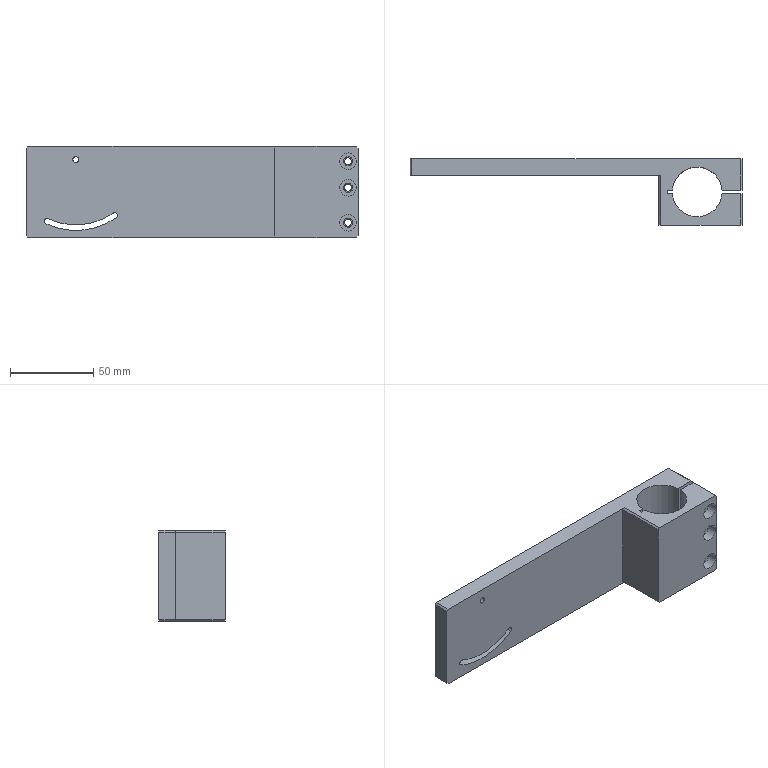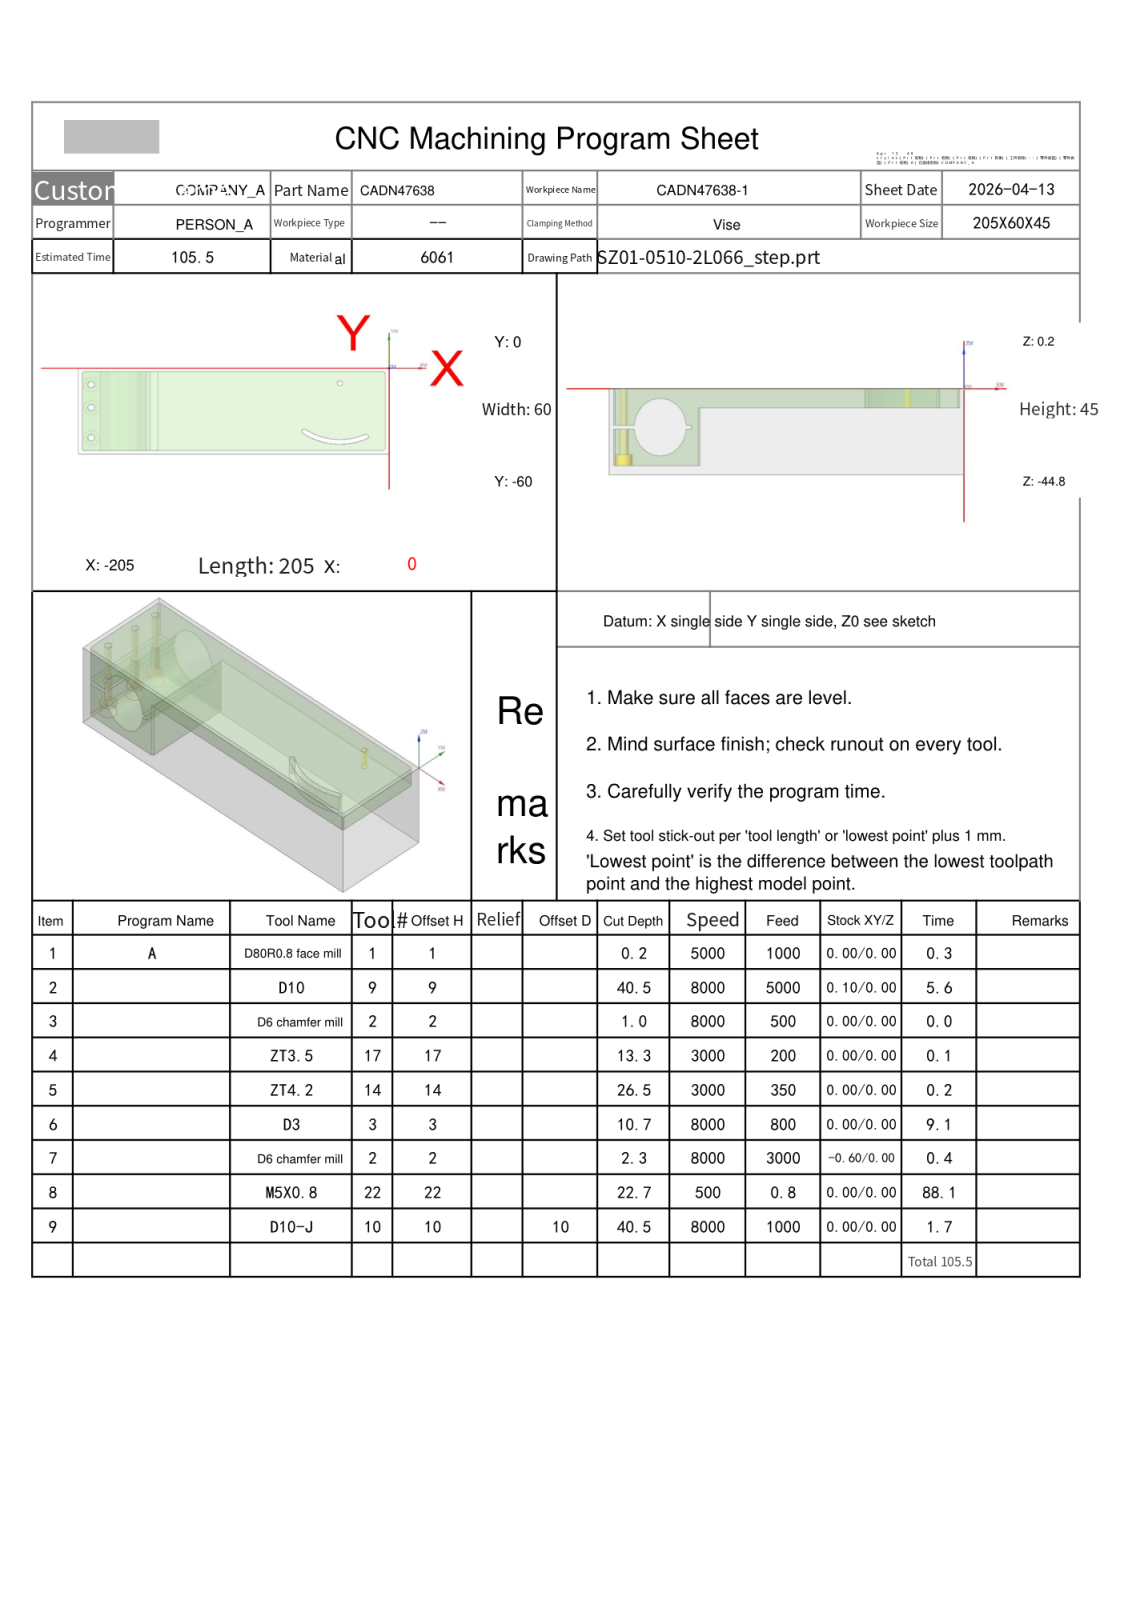NC program | NX | posted by the shop | part box 200 x 40 x 55 mm
Lines 1034 to 2500 of 2500:
N6 T03 M06
(D3  D=3. R=0. H=03 ce=0.10 di=0.00)
(D.N=03 MAX_Z=20. MIN_Z=-10.5 Time=9.14M)
G00 G90 G54 X-36.076 Y-51.374 M03 S8000
G43 H03 Z20.
M08
Z.5
G03 X-15.16 Y-47.686 Z.463 I3.576 J40.874 F800.
G01 X-15.132 Y-47.675
X-15.121 Y-47.646
X-15.136 Y-47.619
X-15.147 Y-47.591
X-15.176 Y-47.581
X-15.202 Y-47.595
G02 X-55.976 Y-44.028 Z.389 I-17.298 J37.095
G01 X-56. Y-44.009
X-56.031 Y-44.014
X-56.046 Y-44.04
X-56.065 Y-44.064
X-56.06 Y-44.094 Z.388
X-56.034 Y-44.11
G03 X-36.076 Y-51.374 Z.351 I23.534 J33.61
X-15.16 Y-47.686 Z.314 I3.576 J40.874
G01 X-15.132 Y-47.675
X-15.121 Y-47.646
X-15.136 Y-47.619
X-15.147 Y-47.591
X-15.176 Y-47.581
X-15.202 Y-47.595
G02 X-55.976 Y-44.028 Z.24 I-17.298 J37.095
G01 X-56. Y-44.009
X-56.031 Y-44.014
X-56.046 Y-44.04
X-56.065 Y-44.064
X-56.06 Y-44.094
X-56.034 Y-44.11
G03 X-36.076 Y-51.374 Z.203 I23.534 J33.61
X-15.16 Y-47.686 Z.166 I3.576 J40.874
G01 X-15.132 Y-47.675
X-15.121 Y-47.646
X-15.136 Y-47.619 Z.165
X-15.147 Y-47.591
X-15.176 Y-47.581
X-15.202 Y-47.595
G02 X-55.976 Y-44.028 Z.091 I-17.298 J37.095
G01 X-56. Y-44.009
X-56.031 Y-44.014
X-56.046 Y-44.04
X-56.065 Y-44.064
X-56.06 Y-44.094
X-56.034 Y-44.11
G03 X-36.076 Y-51.374 Z.054 I23.534 J33.61
X-15.16 Y-47.686 Z.017 I3.576 J40.874
G01 X-15.132 Y-47.675
X-15.121 Y-47.646
X-15.136 Y-47.619
X-15.147 Y-47.591
X-15.176 Y-47.581
X-15.202 Y-47.595
G02 X-55.976 Y-44.028 Z-.057 I-17.298 J37.095
G01 X-56. Y-44.009
X-56.031 Y-44.014
X-56.046 Y-44.04
X-56.065 Y-44.064
X-56.06 Y-44.094
X-56.034 Y-44.11 Z-.058
G03 X-36.076 Y-51.374 Z-.095 I23.534 J33.61
X-15.16 Y-47.686 Z-.132 I3.576 J40.874
G01 X-15.132 Y-47.675
X-15.121 Y-47.646
X-15.136 Y-47.619
X-15.147 Y-47.591
X-15.176 Y-47.581
X-15.202 Y-47.595
G02 X-55.976 Y-44.028 Z-.206 I-17.298 J37.095
G01 X-56. Y-44.009
X-56.031 Y-44.014
X-56.046 Y-44.04
X-56.065 Y-44.064
X-56.06 Y-44.094
X-56.034 Y-44.11
G03 X-36.076 Y-51.374 Z-.243 I23.534 J33.61
X-15.16 Y-47.686 Z-.28 I3.576 J40.874
G01 X-15.132 Y-47.675
X-15.121 Y-47.646
X-15.136 Y-47.619
X-15.147 Y-47.591
X-15.176 Y-47.581 Z-.281
X-15.202 Y-47.595
G02 X-55.976 Y-44.028 Z-.355 I-17.298 J37.095
G01 X-56. Y-44.009
X-56.031 Y-44.014
X-56.046 Y-44.04
X-56.065 Y-44.064
X-56.06 Y-44.094
X-56.034 Y-44.11
G03 X-36.076 Y-51.374 Z-.392 I23.534 J33.61
X-15.16 Y-47.686 Z-.429 I3.576 J40.874
G01 X-15.132 Y-47.675
X-15.121 Y-47.646
X-15.136 Y-47.619
X-15.147 Y-47.591
X-15.176 Y-47.581
X-15.202 Y-47.595
G02 X-55.976 Y-44.028 Z-.503 I-17.298 J37.095
G01 X-56. Y-44.009
X-56.031 Y-44.014
X-56.046 Y-44.04
X-56.065 Y-44.064
X-56.06 Y-44.094
X-56.034 Y-44.11
G03 X-36.076 Y-51.374 Z-.541 I23.534 J33.61
X-15.16 Y-47.686 Z-.578 I3.576 J40.874
G01 X-15.132 Y-47.675
X-15.121 Y-47.646
X-15.136 Y-47.619
X-15.147 Y-47.591
X-15.176 Y-47.581
X-15.202 Y-47.595
G02 X-55.976 Y-44.028 Z-.652 I-17.298 J37.095
G01 X-56. Y-44.009
X-56.031 Y-44.014
X-56.046 Y-44.04
X-56.065 Y-44.064
X-56.06 Y-44.094
X-56.034 Y-44.11
G03 X-36.076 Y-51.374 Z-.689 I23.534 J33.61
X-15.16 Y-47.686 Z-.726 I3.576 J40.874
G01 X-15.132 Y-47.675
X-15.121 Y-47.646
X-15.136 Y-47.619
X-15.147 Y-47.591
X-15.176 Y-47.581
X-15.202 Y-47.595 Z-.727
G02 X-55.976 Y-44.028 Z-.8 I-17.298 J37.095
G01 X-56. Y-44.009 Z-.801
X-56.031 Y-44.014
X-56.046 Y-44.04
X-56.065 Y-44.064
X-56.06 Y-44.094
X-56.034 Y-44.11
G03 X-36.076 Y-51.374 Z-.838 I23.534 J33.61
X-15.16 Y-47.686 Z-.875 I3.576 J40.874
G01 X-15.132 Y-47.675
X-15.121 Y-47.646
X-15.136 Y-47.619
X-15.147 Y-47.591
X-15.176 Y-47.581
X-15.202 Y-47.595
G02 X-55.976 Y-44.028 Z-.949 I-17.298 J37.095
G01 X-56. Y-44.009
X-56.031 Y-44.014
X-56.046 Y-44.04
X-56.065 Y-44.064
X-56.06 Y-44.094
X-56.034 Y-44.11
G03 X-36.076 Y-51.374 Z-.986 I23.534 J33.61
X-15.16 Y-47.686 Z-1.024 I3.576 J40.874
G01 X-15.132 Y-47.675
X-15.121 Y-47.646
X-15.136 Y-47.619
X-15.147 Y-47.591
X-15.176 Y-47.581
X-15.202 Y-47.595
G02 X-55.976 Y-44.028 Z-1.098 I-17.298 J37.095
G01 X-56. Y-44.009
X-56.031 Y-44.014
X-56.046 Y-44.04
X-56.065 Y-44.064
X-56.06 Y-44.094
X-56.034 Y-44.11
G03 X-36.076 Y-51.374 Z-1.135 I23.534 J33.61
X-15.16 Y-47.686 Z-1.172 I3.576 J40.874
G01 X-15.132 Y-47.675
X-15.121 Y-47.646
X-15.136 Y-47.619
X-15.147 Y-47.591
X-15.176 Y-47.581
X-15.202 Y-47.595
G02 X-55.976 Y-44.028 Z-1.246 I-17.298 J37.095
G01 X-56. Y-44.009
X-56.031 Y-44.014 Z-1.247
X-56.046 Y-44.04
X-56.065 Y-44.064
X-56.06 Y-44.094
X-56.034 Y-44.11
G03 X-36.076 Y-51.374 Z-1.284 I23.534 J33.61
X-15.16 Y-47.686 Z-1.321 I3.576 J40.874
G01 X-15.132 Y-47.675
X-15.121 Y-47.646
X-15.136 Y-47.619
X-15.147 Y-47.591
X-15.176 Y-47.581
X-15.202 Y-47.595
G02 X-55.976 Y-44.028 Z-1.395 I-17.298 J37.095
G01 X-56. Y-44.009
X-56.031 Y-44.014
X-56.046 Y-44.04
X-56.065 Y-44.064
X-56.06 Y-44.094
X-56.034 Y-44.11
G03 X-36.076 Y-51.374 Z-1.432 I23.534 J33.61
X-15.16 Y-47.686 Z-1.47 I3.576 J40.874
G01 X-15.132 Y-47.675
X-15.121 Y-47.646
X-15.136 Y-47.619
X-15.147 Y-47.591
X-15.176 Y-47.581
X-15.202 Y-47.595
G02 X-55.976 Y-44.028 Z-1.544 I-17.298 J37.095
G01 X-56. Y-44.009
X-56.031 Y-44.014
X-56.046 Y-44.04
X-56.065 Y-44.064
X-56.06 Y-44.094
X-56.034 Y-44.11
G03 X-36.076 Y-51.374 Z-1.581 I23.534 J33.61
X-15.16 Y-47.686 Z-1.618 I3.576 J40.874
G01 X-15.132 Y-47.675
X-15.121 Y-47.646
X-15.136 Y-47.619
X-15.147 Y-47.591
X-15.176 Y-47.581
X-15.202 Y-47.595
G02 X-55.976 Y-44.028 Z-1.692 I-17.298 J37.095
G01 X-56. Y-44.009
X-56.031 Y-44.014
X-56.046 Y-44.04 Z-1.693
X-56.065 Y-44.064
X-56.06 Y-44.094
X-56.034 Y-44.11
G03 X-36.076 Y-51.374 Z-1.73 I23.534 J33.61
X-15.16 Y-47.686 Z-1.767 I3.576 J40.874
G01 X-15.132 Y-47.675
X-15.121 Y-47.646
X-15.136 Y-47.619
X-15.147 Y-47.591
X-15.176 Y-47.581
X-15.202 Y-47.595
G02 X-55.976 Y-44.028 Z-1.841 I-17.298 J37.095
G01 X-56. Y-44.009
X-56.031 Y-44.014
X-56.046 Y-44.04
X-56.065 Y-44.064
X-56.06 Y-44.094
X-56.034 Y-44.11
G03 X-36.076 Y-51.374 Z-1.878 I23.534 J33.61
X-15.16 Y-47.686 Z-1.915 I3.576 J40.874
G01 X-15.132 Y-47.675
X-15.121 Y-47.646 Z-1.916
X-15.136 Y-47.619
X-15.147 Y-47.591
X-15.176 Y-47.581
X-15.202 Y-47.595
G02 X-55.976 Y-44.028 Z-1.99 I-17.298 J37.095
G01 X-56. Y-44.009
X-56.031 Y-44.014
X-56.046 Y-44.04
X-56.065 Y-44.064
X-56.06 Y-44.094
X-56.034 Y-44.11
G03 X-36.076 Y-51.374 Z-2.027 I23.534 J33.61
X-15.16 Y-47.686 Z-2.064 I3.576 J40.874
G01 X-15.132 Y-47.675
X-15.121 Y-47.646
X-15.136 Y-47.619
X-15.147 Y-47.591
X-15.176 Y-47.581
X-15.202 Y-47.595
G02 X-55.976 Y-44.028 Z-2.138 I-17.298 J37.095
G01 X-56. Y-44.009
X-56.031 Y-44.014
X-56.046 Y-44.04
X-56.065 Y-44.064 Z-2.139
X-56.06 Y-44.094
X-56.034 Y-44.11
G03 X-36.076 Y-51.374 Z-2.176 I23.534 J33.61
X-15.16 Y-47.686 Z-2.213 I3.576 J40.874
G01 X-15.132 Y-47.675
X-15.121 Y-47.646
X-15.136 Y-47.619
X-15.147 Y-47.591
X-15.176 Y-47.581
X-15.202 Y-47.595
G02 X-55.976 Y-44.028 Z-2.287 I-17.298 J37.095
G01 X-56. Y-44.009
X-56.031 Y-44.014
X-56.046 Y-44.04
X-56.065 Y-44.064
X-56.06 Y-44.094
X-56.034 Y-44.11
G03 X-36.076 Y-51.374 Z-2.324 I23.534 J33.61
X-15.16 Y-47.686 Z-2.361 I3.576 J40.874
G01 X-15.132 Y-47.675
X-15.121 Y-47.646
X-15.136 Y-47.619 Z-2.362
X-15.147 Y-47.591
X-15.176 Y-47.581
X-15.202 Y-47.595
G02 X-55.976 Y-44.028 Z-2.436 I-17.298 J37.095
G01 X-56. Y-44.009
X-56.031 Y-44.014
X-56.046 Y-44.04
X-56.065 Y-44.064
X-56.06 Y-44.094
X-56.034 Y-44.11
G03 X-36.076 Y-51.374 Z-2.473 I23.534 J33.61
X-15.16 Y-47.686 Z-2.51 I3.576 J40.874
G01 X-15.132 Y-47.675
X-15.121 Y-47.646
X-15.136 Y-47.619
X-15.147 Y-47.591
X-15.176 Y-47.581
X-15.202 Y-47.595
G02 X-55.976 Y-44.028 Z-2.584 I-17.298 J37.095
G01 X-56. Y-44.009
X-56.031 Y-44.014
X-56.046 Y-44.04
X-56.065 Y-44.064
X-56.06 Y-44.094 Z-2.585
X-56.034 Y-44.11
G03 X-36.076 Y-51.374 Z-2.622 I23.534 J33.61
X-15.16 Y-47.686 Z-2.659 I3.576 J40.874
G01 X-15.132 Y-47.675
X-15.121 Y-47.646
X-15.136 Y-47.619
X-15.147 Y-47.591
X-15.176 Y-47.581
X-15.202 Y-47.595
G02 X-55.976 Y-44.028 Z-2.733 I-17.298 J37.095
G01 X-56. Y-44.009
X-56.031 Y-44.014
X-56.046 Y-44.04
X-56.065 Y-44.064
X-56.06 Y-44.094
X-56.034 Y-44.11
G03 X-36.076 Y-51.374 Z-2.77 I23.534 J33.61
X-15.16 Y-47.686 Z-2.807 I3.576 J40.874
G01 X-15.132 Y-47.675
X-15.121 Y-47.646
X-15.136 Y-47.619
X-15.147 Y-47.591 Z-2.808
X-15.176 Y-47.581
X-15.202 Y-47.595
G02 X-55.976 Y-44.028 Z-2.882 I-17.298 J37.095
G01 X-56. Y-44.009
X-56.031 Y-44.014
X-56.046 Y-44.04
X-56.065 Y-44.064
X-56.06 Y-44.094
X-56.034 Y-44.11
G03 X-36.076 Y-51.374 Z-2.919 I23.534 J33.61
X-15.16 Y-47.686 Z-2.956 I3.576 J40.874
G01 X-15.132 Y-47.675
X-15.121 Y-47.646
X-15.136 Y-47.619
X-15.147 Y-47.591
X-15.176 Y-47.581
X-15.202 Y-47.595
G02 X-55.976 Y-44.028 Z-3.03 I-17.298 J37.095
G01 X-56. Y-44.009
X-56.031 Y-44.014
X-56.046 Y-44.04
X-56.065 Y-44.064
X-56.06 Y-44.094
X-56.034 Y-44.11
G03 X-36.076 Y-51.374 Z-3.068 I23.534 J33.61
X-15.16 Y-47.686 Z-3.105 I3.576 J40.874
G01 X-15.132 Y-47.675
X-15.121 Y-47.646
X-15.136 Y-47.619
X-15.147 Y-47.591
X-15.176 Y-47.581
X-15.202 Y-47.595
G02 X-55.976 Y-44.028 Z-3.179 I-17.298 J37.095
G01 X-56. Y-44.009
X-56.031 Y-44.014
X-56.046 Y-44.04
X-56.065 Y-44.064
X-56.06 Y-44.094
X-56.034 Y-44.11
G03 X-36.076 Y-51.374 Z-3.216 I23.534 J33.61
X-15.16 Y-47.686 Z-3.253 I3.576 J40.874
G01 X-15.132 Y-47.675
X-15.121 Y-47.646
X-15.136 Y-47.619
X-15.147 Y-47.591
X-15.176 Y-47.581 Z-3.254
X-15.202 Y-47.595
G02 X-55.976 Y-44.028 Z-3.328 I-17.298 J37.095
G01 X-56. Y-44.009
X-56.031 Y-44.014
X-56.046 Y-44.04
X-56.065 Y-44.064
X-56.06 Y-44.094
X-56.034 Y-44.11
G03 X-36.076 Y-51.374 Z-3.365 I23.534 J33.61
X-15.16 Y-47.686 Z-3.402 I3.576 J40.874
G01 X-15.132 Y-47.675
X-15.121 Y-47.646
X-15.136 Y-47.619
X-15.147 Y-47.591
X-15.176 Y-47.581
X-15.202 Y-47.595
G02 X-55.976 Y-44.028 Z-3.476 I-17.298 J37.095
G01 X-56. Y-44.009
X-56.031 Y-44.014
X-56.046 Y-44.04
X-56.065 Y-44.064
X-56.06 Y-44.094
X-56.034 Y-44.11
G03 X-36.076 Y-51.374 Z-3.514 I23.534 J33.61
X-15.16 Y-47.686 Z-3.551 I3.576 J40.874
G01 X-15.132 Y-47.675
X-15.121 Y-47.646
X-15.136 Y-47.619
X-15.147 Y-47.591
X-15.176 Y-47.581
X-15.202 Y-47.595
G02 X-55.976 Y-44.028 Z-3.625 I-17.298 J37.095
G01 X-56. Y-44.009
X-56.031 Y-44.014
X-56.046 Y-44.04
X-56.065 Y-44.064
X-56.06 Y-44.094
X-56.034 Y-44.11
G03 X-36.076 Y-51.374 Z-3.662 I23.534 J33.61
X-15.16 Y-47.686 Z-3.699 I3.576 J40.874
G01 X-15.132 Y-47.675
X-15.121 Y-47.646
X-15.136 Y-47.619
X-15.147 Y-47.591
X-15.176 Y-47.581
X-15.202 Y-47.595 Z-3.7
G02 X-55.976 Y-44.028 Z-3.773 I-17.298 J37.095
G01 X-56. Y-44.009 Z-3.774
X-56.031 Y-44.014
X-56.046 Y-44.04
X-56.065 Y-44.064
X-56.06 Y-44.094
X-56.034 Y-44.11
G03 X-36.076 Y-51.374 Z-3.811 I23.534 J33.61
X-15.16 Y-47.686 Z-3.848 I3.576 J40.874
G01 X-15.132 Y-47.675
X-15.121 Y-47.646
X-15.136 Y-47.619
X-15.147 Y-47.591
X-15.176 Y-47.581
X-15.202 Y-47.595
G02 X-55.976 Y-44.028 Z-3.922 I-17.298 J37.095
G01 X-56. Y-44.009
X-56.031 Y-44.014
X-56.046 Y-44.04
X-56.065 Y-44.064
X-56.06 Y-44.094
X-56.034 Y-44.11
G03 X-36.076 Y-51.374 Z-3.959 I23.534 J33.61
X-15.16 Y-47.686 Z-3.997 I3.576 J40.874
G01 X-15.132 Y-47.675
X-15.121 Y-47.646
X-15.136 Y-47.619
X-15.147 Y-47.591
X-15.176 Y-47.581
X-15.202 Y-47.595
G02 X-55.976 Y-44.028 Z-4.071 I-17.298 J37.095
G01 X-56. Y-44.009
X-56.031 Y-44.014
X-56.046 Y-44.04
X-56.065 Y-44.064
X-56.06 Y-44.094
X-56.034 Y-44.11
G03 X-36.076 Y-51.374 Z-4.108 I23.534 J33.61
X-15.16 Y-47.686 Z-4.145 I3.576 J40.874
G01 X-15.132 Y-47.675
X-15.121 Y-47.646
X-15.136 Y-47.619
X-15.147 Y-47.591
X-15.176 Y-47.581
X-15.202 Y-47.595
G02 X-55.976 Y-44.028 Z-4.219 I-17.298 J37.095
G01 X-56. Y-44.009
X-56.031 Y-44.014 Z-4.22
X-56.046 Y-44.04
X-56.065 Y-44.064
X-56.06 Y-44.094
X-56.034 Y-44.11
G03 X-36.076 Y-51.374 Z-4.257 I23.534 J33.61
X-15.16 Y-47.686 Z-4.294 I3.576 J40.874
G01 X-15.132 Y-47.675
X-15.121 Y-47.646
X-15.136 Y-47.619
X-15.147 Y-47.591
X-15.176 Y-47.581
X-15.202 Y-47.595
G02 X-55.976 Y-44.028 Z-4.368 I-17.298 J37.095
G01 X-56. Y-44.009
X-56.031 Y-44.014
X-56.046 Y-44.04
X-56.065 Y-44.064
X-56.06 Y-44.094
X-56.034 Y-44.11
G03 X-36.076 Y-51.374 Z-4.405 I23.534 J33.61
X-15.16 Y-47.686 Z-4.442 I3.576 J40.874
G01 X-15.132 Y-47.675 Z-4.443
X-15.121 Y-47.646
X-15.136 Y-47.619
X-15.147 Y-47.591
X-15.176 Y-47.581
X-15.202 Y-47.595
G02 X-55.976 Y-44.028 Z-4.517 I-17.298 J37.095
G01 X-56. Y-44.009
X-56.031 Y-44.014
X-56.046 Y-44.04
X-56.065 Y-44.064
X-56.06 Y-44.094
X-56.034 Y-44.11
G03 X-36.076 Y-51.374 Z-4.554 I23.534 J33.61
X-15.16 Y-47.686 Z-4.591 I3.576 J40.874
G01 X-15.132 Y-47.675
X-15.121 Y-47.646
X-15.136 Y-47.619
X-15.147 Y-47.591
X-15.176 Y-47.581
X-15.202 Y-47.595
G02 X-55.976 Y-44.028 Z-4.665 I-17.298 J37.095
G01 X-56. Y-44.009
X-56.031 Y-44.014
X-56.046 Y-44.04
X-56.065 Y-44.064 Z-4.666
X-56.06 Y-44.094
X-56.034 Y-44.11
G03 X-36.076 Y-51.374 Z-4.703 I23.534 J33.61
X-15.16 Y-47.686 Z-4.74 I3.576 J40.874
G01 X-15.132 Y-47.675
X-15.121 Y-47.646
X-15.136 Y-47.619
X-15.147 Y-47.591
X-15.176 Y-47.581
X-15.202 Y-47.595
G02 X-55.976 Y-44.028 Z-4.814 I-17.298 J37.095
G01 X-56. Y-44.009
X-56.031 Y-44.014
X-56.046 Y-44.04
X-56.065 Y-44.064
X-56.06 Y-44.094
X-56.034 Y-44.11
G03 X-36.076 Y-51.374 Z-4.851 I23.534 J33.61
X-15.16 Y-47.686 Z-4.888 I3.576 J40.874
G01 X-15.132 Y-47.675
X-15.121 Y-47.646 Z-4.889
X-15.136 Y-47.619
X-15.147 Y-47.591
X-15.176 Y-47.581
X-15.202 Y-47.595
G02 X-55.976 Y-44.028 Z-4.963 I-17.298 J37.095
G01 X-56. Y-44.009
X-56.031 Y-44.014
X-56.046 Y-44.04
X-56.065 Y-44.064
X-56.06 Y-44.094
X-56.034 Y-44.11
G03 X-36.076 Y-51.374 Z-5. I23.534 J33.61
X-15.16 Y-47.686 Z-5.037 I3.576 J40.874
G01 X-15.132 Y-47.675
X-15.121 Y-47.646
X-15.136 Y-47.619
X-15.147 Y-47.591
X-15.176 Y-47.581
X-15.202 Y-47.595
G02 X-55.976 Y-44.028 Z-5.111 I-17.298 J37.095
G01 X-56. Y-44.009
X-56.031 Y-44.014
X-56.046 Y-44.04
X-56.065 Y-44.064
X-56.06 Y-44.094 Z-5.112
X-56.034 Y-44.11
G03 X-36.076 Y-51.374 Z-5.149 I23.534 J33.61
X-15.16 Y-47.686 Z-5.186 I3.576 J40.874
G01 X-15.132 Y-47.675
X-15.121 Y-47.646
X-15.136 Y-47.619
X-15.147 Y-47.591
X-15.176 Y-47.581
X-15.202 Y-47.595
G02 X-55.976 Y-44.028 Z-5.26 I-17.298 J37.095
G01 X-56. Y-44.009
X-56.031 Y-44.014
X-56.046 Y-44.04
X-56.065 Y-44.064
X-56.06 Y-44.094
X-56.034 Y-44.11
G03 X-36.076 Y-51.374 Z-5.297 I23.534 J33.61
X-15.16 Y-47.686 Z-5.334 I3.576 J40.874
G01 X-15.132 Y-47.675
X-15.121 Y-47.646
X-15.136 Y-47.619 Z-5.335
X-15.147 Y-47.591
X-15.176 Y-47.581
X-15.202 Y-47.595
G02 X-55.976 Y-44.028 Z-5.409 I-17.298 J37.095
G01 X-56. Y-44.009
X-56.031 Y-44.014
X-56.046 Y-44.04
X-56.065 Y-44.064
X-56.06 Y-44.094
X-56.034 Y-44.11
G03 X-36.076 Y-51.374 Z-5.446 I23.534 J33.61
X-15.16 Y-47.686 Z-5.483 I3.576 J40.874
G01 X-15.132 Y-47.675
X-15.121 Y-47.646
X-15.136 Y-47.619
X-15.147 Y-47.591
X-15.176 Y-47.581
X-15.202 Y-47.595
G02 X-55.976 Y-44.028 Z-5.557 I-17.298 J37.095
G01 X-56. Y-44.009
X-56.031 Y-44.014
X-56.046 Y-44.04
X-56.065 Y-44.064
X-56.06 Y-44.094
X-56.034 Y-44.11 Z-5.558
G03 X-36.076 Y-51.374 Z-5.595 I23.534 J33.61
X-15.16 Y-47.686 Z-5.632 I3.576 J40.874
G01 X-15.132 Y-47.675
X-15.121 Y-47.646
X-15.136 Y-47.619
X-15.147 Y-47.591
X-15.176 Y-47.581
X-15.202 Y-47.595
G02 X-55.976 Y-44.028 Z-5.706 I-17.298 J37.095
G01 X-56. Y-44.009
X-56.031 Y-44.014
X-56.046 Y-44.04
X-56.065 Y-44.064
X-56.06 Y-44.094
X-56.034 Y-44.11
G03 X-36.076 Y-51.374 Z-5.743 I23.534 J33.61
X-15.16 Y-47.686 Z-5.78 I3.576 J40.874
G01 X-15.132 Y-47.675
X-15.121 Y-47.646
X-15.136 Y-47.619
X-15.147 Y-47.591
X-15.176 Y-47.581 Z-5.781
X-15.202 Y-47.595
G02 X-55.976 Y-44.028 Z-5.855 I-17.298 J37.095
G01 X-56. Y-44.009
X-56.031 Y-44.014
X-56.046 Y-44.04
X-56.065 Y-44.064
X-56.06 Y-44.094
X-56.034 Y-44.11
G03 X-36.076 Y-51.374 Z-5.892 I23.534 J33.61
X-15.16 Y-47.686 Z-5.929 I3.576 J40.874
G01 X-15.132 Y-47.675
X-15.121 Y-47.646
X-15.136 Y-47.619
X-15.147 Y-47.591
X-15.176 Y-47.581
X-15.202 Y-47.595
G02 X-55.976 Y-44.028 Z-6.003 I-17.298 J37.095
G01 X-56. Y-44.009
X-56.031 Y-44.014
X-56.046 Y-44.04
X-56.065 Y-44.064
X-56.06 Y-44.094
X-56.034 Y-44.11
G03 X-36.076 Y-51.374 Z-6.041 I23.534 J33.61
X-15.16 Y-47.686 Z-6.078 I3.576 J40.874
G01 X-15.132 Y-47.675
X-15.121 Y-47.646
X-15.136 Y-47.619
X-15.147 Y-47.591
X-15.176 Y-47.581
X-15.202 Y-47.595
G02 X-55.976 Y-44.028 Z-6.152 I-17.298 J37.095
G01 X-56. Y-44.009
X-56.031 Y-44.014
X-56.046 Y-44.04
X-56.065 Y-44.064
X-56.06 Y-44.094
X-56.034 Y-44.11
G03 X-36.076 Y-51.374 Z-6.189 I23.534 J33.61
X-15.16 Y-47.686 Z-6.226 I3.576 J40.874
G01 X-15.132 Y-47.675
X-15.121 Y-47.646
X-15.136 Y-47.619
X-15.147 Y-47.591
X-15.176 Y-47.581
X-15.202 Y-47.595 Z-6.227
G02 X-55.976 Y-44.028 Z-6.3 I-17.298 J37.095
G01 X-56. Y-44.009 Z-6.301
X-56.031 Y-44.014
X-56.046 Y-44.04
X-56.065 Y-44.064
X-56.06 Y-44.094
X-56.034 Y-44.11
G03 X-36.076 Y-51.374 Z-6.338 I23.534 J33.61
X-15.16 Y-47.686 Z-6.375 I3.576 J40.874
G01 X-15.132 Y-47.675
X-15.121 Y-47.646
X-15.136 Y-47.619
X-15.147 Y-47.591
X-15.176 Y-47.581
X-15.202 Y-47.595
G02 X-55.976 Y-44.028 Z-6.449 I-17.298 J37.095
G01 X-56. Y-44.009
X-56.031 Y-44.014
X-56.046 Y-44.04
X-56.065 Y-44.064
X-56.06 Y-44.094
X-56.034 Y-44.11
G03 X-36.076 Y-51.374 Z-6.486 I23.534 J33.61
X-15.16 Y-47.686 Z-6.524 I3.576 J40.874
G01 X-15.132 Y-47.675
X-15.121 Y-47.646
X-15.136 Y-47.619
X-15.147 Y-47.591
X-15.176 Y-47.581
X-15.202 Y-47.595
G02 X-55.976 Y-44.028 Z-6.598 I-17.298 J37.095
G01 X-56. Y-44.009
X-56.031 Y-44.014
X-56.046 Y-44.04
X-56.065 Y-44.064
X-56.06 Y-44.094
X-56.034 Y-44.11
G03 X-36.076 Y-51.374 Z-6.635 I23.534 J33.61
X-15.16 Y-47.686 Z-6.672 I3.576 J40.874
G01 X-15.132 Y-47.675
X-15.121 Y-47.646
X-15.136 Y-47.619
X-15.147 Y-47.591
X-15.176 Y-47.581
X-15.202 Y-47.595
G02 X-55.976 Y-44.028 Z-6.746 I-17.298 J37.095
G01 X-56. Y-44.009
X-56.031 Y-44.014 Z-6.747
X-56.046 Y-44.04
X-56.065 Y-44.064
X-56.06 Y-44.094
X-56.034 Y-44.11
G03 X-36.076 Y-51.374 Z-6.784 I23.534 J33.61
X-15.16 Y-47.686 Z-6.821 I3.576 J40.874
G01 X-15.132 Y-47.675
X-15.121 Y-47.646
X-15.136 Y-47.619
X-15.147 Y-47.591
X-15.176 Y-47.581
X-15.202 Y-47.595
G02 X-55.976 Y-44.028 Z-6.895 I-17.298 J37.095
G01 X-56. Y-44.009
X-56.031 Y-44.014
X-56.046 Y-44.04
X-56.065 Y-44.064
X-56.06 Y-44.094
X-56.034 Y-44.11
G03 X-36.076 Y-51.374 Z-6.932 I23.534 J33.61
X-15.16 Y-47.686 Z-6.97 I3.576 J40.874
G01 X-15.132 Y-47.675
X-15.121 Y-47.646
X-15.136 Y-47.619
X-15.147 Y-47.591
X-15.176 Y-47.581
X-15.202 Y-47.595
G02 X-55.976 Y-44.028 Z-7.044 I-17.298 J37.095
G01 X-56. Y-44.009
X-56.031 Y-44.014
X-56.046 Y-44.04
X-56.065 Y-44.064
X-56.06 Y-44.094
X-56.034 Y-44.11
G03 X-36.076 Y-51.374 Z-7.081 I23.534 J33.61
X-15.16 Y-47.686 Z-7.118 I3.576 J40.874
G01 X-15.132 Y-47.675
X-15.121 Y-47.646
X-15.136 Y-47.619
X-15.147 Y-47.591
X-15.176 Y-47.581
X-15.202 Y-47.595
G02 X-55.976 Y-44.028 Z-7.192 I-17.298 J37.095
G01 X-56. Y-44.009
X-56.031 Y-44.014
X-56.046 Y-44.04 Z-7.193
X-56.065 Y-44.064
X-56.06 Y-44.094
X-56.034 Y-44.11
G03 X-36.076 Y-51.374 Z-7.23 I23.534 J33.61
X-15.16 Y-47.686 Z-7.267 I3.576 J40.874
G01 X-15.132 Y-47.675
X-15.121 Y-47.646
X-15.136 Y-47.619
X-15.147 Y-47.591
X-15.176 Y-47.581
X-15.202 Y-47.595
G02 X-55.976 Y-44.028 Z-7.341 I-17.298 J37.095
G01 X-56. Y-44.009
X-56.031 Y-44.014
X-56.046 Y-44.04
X-56.065 Y-44.064
X-56.06 Y-44.094
X-56.034 Y-44.11
G03 X-36.076 Y-51.374 Z-7.378 I23.534 J33.61
X-15.16 Y-47.686 Z-7.415 I3.576 J40.874
G01 X-15.132 Y-47.675
X-15.121 Y-47.646 Z-7.416
X-15.136 Y-47.619
X-15.147 Y-47.591
X-15.176 Y-47.581
X-15.202 Y-47.595
G02 X-55.976 Y-44.028 Z-7.49 I-17.298 J37.095
G01 X-56. Y-44.009
X-56.031 Y-44.014
X-56.046 Y-44.04
X-56.065 Y-44.064
X-56.06 Y-44.094
X-56.034 Y-44.11
G03 X-36.076 Y-51.374 Z-7.527 I23.534 J33.61
X-15.16 Y-47.686 Z-7.564 I3.576 J40.874
G01 X-15.132 Y-47.675
X-15.121 Y-47.646
X-15.136 Y-47.619
X-15.147 Y-47.591
X-15.176 Y-47.581
X-15.202 Y-47.595
G02 X-55.976 Y-44.028 Z-7.638 I-17.298 J37.095
G01 X-56. Y-44.009
X-56.031 Y-44.014
X-56.046 Y-44.04
X-56.065 Y-44.064 Z-7.639
X-56.06 Y-44.094
X-56.034 Y-44.11
G03 X-36.076 Y-51.374 Z-7.676 I23.534 J33.61
X-15.16 Y-47.686 Z-7.713 I3.576 J40.874
G01 X-15.132 Y-47.675
X-15.121 Y-47.646
X-15.136 Y-47.619
X-15.147 Y-47.591
X-15.176 Y-47.581
X-15.202 Y-47.595
G02 X-55.976 Y-44.028 Z-7.787 I-17.298 J37.095
G01 X-56. Y-44.009
X-56.031 Y-44.014
X-56.046 Y-44.04
X-56.065 Y-44.064
X-56.06 Y-44.094
X-56.034 Y-44.11
G03 X-36.076 Y-51.374 Z-7.824 I23.534 J33.61
X-15.16 Y-47.686 Z-7.861 I3.576 J40.874
G01 X-15.132 Y-47.675
X-15.121 Y-47.646
X-15.136 Y-47.619 Z-7.862
X-15.147 Y-47.591
X-15.176 Y-47.581
X-15.202 Y-47.595
G02 X-55.976 Y-44.028 Z-7.936 I-17.298 J37.095
G01 X-56. Y-44.009
X-56.031 Y-44.014
X-56.046 Y-44.04
X-56.065 Y-44.064
X-56.06 Y-44.094
X-56.034 Y-44.11
G03 X-36.076 Y-51.374 Z-7.973 I23.534 J33.61
X-15.16 Y-47.686 Z-8.01 I3.576 J40.874
G01 X-15.132 Y-47.675
X-15.121 Y-47.646
X-15.136 Y-47.619
X-15.147 Y-47.591
X-15.176 Y-47.581
X-15.202 Y-47.595
G02 X-55.976 Y-44.028 Z-8.084 I-17.298 J37.095
G01 X-56. Y-44.009
X-56.031 Y-44.014
X-56.046 Y-44.04
X-56.065 Y-44.064
X-56.06 Y-44.094 Z-8.085
X-56.034 Y-44.11
G03 X-36.076 Y-51.374 Z-8.122 I23.534 J33.61
X-15.16 Y-47.686 Z-8.159 I3.576 J40.874
G01 X-15.132 Y-47.675
X-15.121 Y-47.646
X-15.136 Y-47.619
X-15.147 Y-47.591
X-15.176 Y-47.581
X-15.202 Y-47.595
G02 X-55.976 Y-44.028 Z-8.233 I-17.298 J37.095
G01 X-56. Y-44.009
X-56.031 Y-44.014
X-56.046 Y-44.04
X-56.065 Y-44.064
X-56.06 Y-44.094
X-56.034 Y-44.11
G03 X-36.076 Y-51.374 Z-8.27 I23.534 J33.61
X-15.16 Y-47.686 Z-8.307 I3.576 J40.874
G01 X-15.132 Y-47.675
X-15.121 Y-47.646
X-15.136 Y-47.619
X-15.147 Y-47.591 Z-8.308
X-15.176 Y-47.581
X-15.202 Y-47.595
G02 X-55.976 Y-44.028 Z-8.382 I-17.298 J37.095
G01 X-56. Y-44.009
X-56.031 Y-44.014
X-56.046 Y-44.04
X-56.065 Y-44.064
X-56.06 Y-44.094
X-56.034 Y-44.11
G03 X-36.076 Y-51.374 Z-8.419 I23.534 J33.61
X-15.16 Y-47.686 Z-8.456 I3.576 J40.874
G01 X-15.132 Y-47.675
X-15.121 Y-47.646
X-15.136 Y-47.619
X-15.147 Y-47.591
X-15.176 Y-47.581
X-15.202 Y-47.595
G02 X-55.976 Y-44.028 Z-8.53 I-17.298 J37.095
G01 X-56. Y-44.009
X-56.031 Y-44.014
X-56.046 Y-44.04
X-56.065 Y-44.064
X-56.06 Y-44.094
X-56.034 Y-44.11
G03 X-36.076 Y-51.374 Z-8.568 I23.534 J33.61
X-15.16 Y-47.686 Z-8.605 I3.576 J40.874
G01 X-15.132 Y-47.675
X-15.121 Y-47.646
X-15.136 Y-47.619
X-15.147 Y-47.591
X-15.176 Y-47.581
X-15.202 Y-47.595
G02 X-55.976 Y-44.028 Z-8.679 I-17.298 J37.095
G01 X-56. Y-44.009
X-56.031 Y-44.014
X-56.046 Y-44.04
X-56.065 Y-44.064
X-56.06 Y-44.094
X-56.034 Y-44.11
G03 X-36.076 Y-51.374 Z-8.716 I23.534 J33.61
X-15.16 Y-47.686 Z-8.753 I3.576 J40.874
G01 X-15.132 Y-47.675
X-15.121 Y-47.646
X-15.136 Y-47.619
X-15.147 Y-47.591
X-15.176 Y-47.581 Z-8.754
X-15.202 Y-47.595
G02 X-55.976 Y-44.028 Z-8.828 I-17.298 J37.095
G01 X-56. Y-44.009
X-56.031 Y-44.014
X-56.046 Y-44.04
X-56.065 Y-44.064
X-56.06 Y-44.094
X-56.034 Y-44.11
G03 X-36.076 Y-51.374 Z-8.865 I23.534 J33.61
X-15.16 Y-47.686 Z-8.902 I3.576 J40.874
G01 X-15.132 Y-47.675
X-15.121 Y-47.646
X-15.136 Y-47.619
X-15.147 Y-47.591
X-15.176 Y-47.581
X-15.202 Y-47.595
G02 X-55.976 Y-44.028 Z-8.976 I-17.298 J37.095
G01 X-56. Y-44.009
X-56.031 Y-44.014
X-56.046 Y-44.04
X-56.065 Y-44.064
X-56.06 Y-44.094
X-56.034 Y-44.11
G03 X-36.076 Y-51.374 Z-9.014 I23.534 J33.61
X-15.16 Y-47.686 Z-9.051 I3.576 J40.874
G01 X-15.132 Y-47.675
X-15.121 Y-47.646
X-15.136 Y-47.619
X-15.147 Y-47.591
X-15.176 Y-47.581
X-15.202 Y-47.595
G02 X-55.976 Y-44.028 Z-9.125 I-17.298 J37.095
G01 X-56. Y-44.009
X-56.031 Y-44.014
X-56.046 Y-44.04
X-56.065 Y-44.064
X-56.06 Y-44.094
X-56.034 Y-44.11
G03 X-36.076 Y-51.374 Z-9.162 I23.534 J33.61
X-15.16 Y-47.686 Z-9.199 I3.576 J40.874
G01 X-15.132 Y-47.675
X-15.121 Y-47.646
X-15.136 Y-47.619
X-15.147 Y-47.591
X-15.176 Y-47.581
X-15.202 Y-47.595 Z-9.2
G02 X-55.976 Y-44.028 Z-9.273 I-17.298 J37.095
G01 X-56. Y-44.009 Z-9.274
X-56.031 Y-44.014
X-56.046 Y-44.04
X-56.065 Y-44.064
X-56.06 Y-44.094
X-56.034 Y-44.11
G03 X-36.076 Y-51.374 Z-9.311 I23.534 J33.61
X-15.16 Y-47.686 Z-9.348 I3.576 J40.874
G01 X-15.132 Y-47.675
X-15.121 Y-47.646
X-15.136 Y-47.619
X-15.147 Y-47.591
X-15.176 Y-47.581
X-15.202 Y-47.595
G02 X-55.976 Y-44.028 Z-9.422 I-17.298 J37.095
G01 X-56. Y-44.009
X-56.031 Y-44.014
X-56.046 Y-44.04
X-56.065 Y-44.064
X-56.06 Y-44.094
X-56.034 Y-44.11
G03 X-36.076 Y-51.374 Z-9.459 I23.534 J33.61
X-15.16 Y-47.686 Z-9.497 I3.576 J40.874
G01 X-15.132 Y-47.675
X-15.121 Y-47.646
X-15.136 Y-47.619
X-15.147 Y-47.591
X-15.176 Y-47.581
X-15.202 Y-47.595
G02 X-55.976 Y-44.028 Z-9.571 I-17.298 J37.095
G01 X-56. Y-44.009
X-56.031 Y-44.014
X-56.046 Y-44.04
X-56.065 Y-44.064
X-56.06 Y-44.094
X-56.034 Y-44.11
G03 X-36.076 Y-51.374 Z-9.608 I23.534 J33.61
X-15.16 Y-47.686 Z-9.645 I3.576 J40.874
G01 X-15.132 Y-47.675
X-15.121 Y-47.646
X-15.136 Y-47.619
X-15.147 Y-47.591
X-15.176 Y-47.581
X-15.202 Y-47.595
G02 X-55.976 Y-44.028 Z-9.719 I-17.298 J37.095
G01 X-56. Y-44.009
X-56.031 Y-44.014 Z-9.72
X-56.046 Y-44.04
X-56.065 Y-44.064
X-56.06 Y-44.094
X-56.034 Y-44.11
G03 X-36.076 Y-51.374 Z-9.757 I23.534 J33.61
X-15.16 Y-47.686 Z-9.794 I3.576 J40.874
G01 X-15.132 Y-47.675
X-15.121 Y-47.646
X-15.136 Y-47.619
X-15.147 Y-47.591
X-15.176 Y-47.581
X-15.202 Y-47.595
G02 X-55.976 Y-44.028 Z-9.868 I-17.298 J37.095
G01 X-56. Y-44.009
X-56.031 Y-44.014
X-56.046 Y-44.04
X-56.065 Y-44.064
X-56.06 Y-44.094
X-56.034 Y-44.11
G03 X-36.076 Y-51.374 Z-9.905 I23.534 J33.61
X-15.16 Y-47.686 Z-9.942 I3.576 J40.874
G01 X-15.132 Y-47.675 Z-9.943
X-15.121 Y-47.646
X-15.136 Y-47.619
X-15.147 Y-47.591
X-15.176 Y-47.581
X-15.202 Y-47.595
G02 X-55.976 Y-44.028 Z-10.017 I-17.298 J37.095
G01 X-56. Y-44.009
X-56.031 Y-44.014
X-56.046 Y-44.04
X-56.065 Y-44.064
X-56.06 Y-44.094
X-56.034 Y-44.11
G03 X-36.076 Y-51.374 Z-10.054 I23.534 J33.61
X-15.16 Y-47.686 Z-10.091 I3.576 J40.874
G01 X-15.132 Y-47.675
X-15.121 Y-47.646
X-15.136 Y-47.619
X-15.147 Y-47.591
X-15.176 Y-47.581
X-15.202 Y-47.595
G02 X-55.976 Y-44.028 Z-10.165 I-17.298 J37.095
G01 X-56. Y-44.009
X-56.031 Y-44.014
X-56.046 Y-44.04
X-56.065 Y-44.064 Z-10.166
X-56.06 Y-44.094
X-56.034 Y-44.11
G03 X-36.076 Y-51.374 Z-10.203 I23.534 J33.61
X-15.16 Y-47.686 Z-10.24 I3.576 J40.874
G01 X-15.132 Y-47.675
X-15.121 Y-47.646
X-15.136 Y-47.619
X-15.147 Y-47.591
X-15.176 Y-47.581
X-15.202 Y-47.595
G02 X-55.976 Y-44.028 Z-10.314 I-17.298 J37.095
G01 X-56. Y-44.009
X-56.031 Y-44.014
X-56.046 Y-44.04
X-56.065 Y-44.064
X-56.06 Y-44.094
X-56.034 Y-44.11
G03 X-36.076 Y-51.374 Z-10.351 I23.534 J33.61
X-15.16 Y-47.686 Z-10.388 I3.576 J40.874
G01 X-15.132 Y-47.675
X-15.121 Y-47.646 Z-10.389
X-15.136 Y-47.619
X-15.147 Y-47.591
X-15.176 Y-47.581
X-15.202 Y-47.595
G02 X-55.976 Y-44.028 Z-10.463 I-17.298 J37.095
G01 X-56. Y-44.009
X-56.031 Y-44.014
X-56.046 Y-44.04
X-56.065 Y-44.064
X-56.06 Y-44.094
X-56.034 Y-44.11
G03 X-36.076 Y-51.374 Z-10.5 I23.534 J33.61
X-32.5 Y-51.53 I3.576 J40.874
X-15.16 Y-47.686 I0.0 J41.03
G01 X-15.121 Y-47.646
X-15.147 Y-47.591
X-15.202 Y-47.595
G02 X-32.5 Y-51.43 I-17.298 J37.095
X-55.976 Y-44.028 I0.0 J40.93
G01 X-56.031 Y-44.014
X-56.065 Y-44.064
X-56.034 Y-44.11
G03 X-36.076 Y-51.374 I23.534 J33.61
X-35.578 Y-51.414 I3.576 J40.874
G01 Z-9.5
G00 Z20.
G00 G90 X-50.426 Y-47.512 M03 S8000
Z20.
Z.5
G01 X-48.873 Y-48.241 Z.04 F300.
X-46.587 Y-49.153 Z-.619
X-44.251 Y-49.926 Z-1.279
X-41.872 Y-50.558 Z-1.938
X-39.46 Y-51.047 Z-2.598
X-37.023 Y-51.391 Z-3.257
X-36.12 Y-51.47 Z-3.5
X-36.117 Y-51.435
G41 D03
X-36.085 Y-51.473
G03 X-32.5 Y-51.63 I3.585 J40.973
X-15.118 Y-47.776 I0.0 J41.13
G01 X-15.031 Y-47.64
G03 X-15.181 Y-47.49 I-.15 J0.0
G01 X-15.244 Y-47.505
G02 X-32.5 Y-51.33 I-17.256 J37.005
X-55.919 Y-43.946 I0.0 J40.83
G01 X-56.005 Y-43.919
G03 X-56.155 Y-44.069 I0.0 J-.15
G01 X-56.091 Y-44.192
G03 X-36.085 Y-51.473 I23.591 J33.692
X-35.586 Y-51.514 I3.585 J40.973
G01 X-35.571 Y-51.515
G03 X-35.372 Y-51.33 I0.0 J.2
G01 G40 X-35.368 Y-51.28
Z-3.
G00 Z20.
X-50.426 Y-47.512
Z-3.
G01 X-48.873 Y-48.241 Z-3.46
X-46.587 Y-49.153 Z-4.119
X-44.251 Y-49.926 Z-4.779
X-41.872 Y-50.558 Z-5.438
X-39.46 Y-51.047 Z-6.098
X-37.023 Y-51.391 Z-6.757
X-36.12 Y-51.47 Z-7.
X-36.117 Y-51.435
G41 D03
X-36.085 Y-51.473
G03 X-32.5 Y-51.63 I3.585 J40.973
X-15.118 Y-47.776 I0.0 J41.13
G01 X-15.031 Y-47.64
G03 X-15.181 Y-47.49 I-.15 J0.0
G01 X-15.244 Y-47.505
G02 X-32.5 Y-51.33 I-17.256 J37.005
X-55.919 Y-43.946 I0.0 J40.83
G01 X-56.005 Y-43.919
G03 X-56.155 Y-44.069 I0.0 J-.15
G01 X-56.091 Y-44.192
G03 X-36.085 Y-51.473 I23.591 J33.692
X-35.586 Y-51.514 I3.585 J40.973
G01 X-35.571 Y-51.515
G03 X-35.372 Y-51.33 I0.0 J.2
G01 G40 X-35.368 Y-51.28
Z-6.5
G00 Z20.
X-50.423 Y-47.474
Z-6.5
G01 X-48.859 Y-48.209 Z-6.963
X-46.575 Y-49.12 Z-7.622
X-44.241 Y-49.892 Z-8.281
X-41.865 Y-50.524 Z-8.939
X-39.455 Y-51.012 Z-9.598
X-37.02 Y-51.355 Z-10.257
X-36.117 Y-51.435 Z-10.5
G41 D03
X-36.085 Y-51.473
G03 X-32.5 Y-51.63 I3.585 J40.973
X-15.118 Y-47.776 I0.0 J41.13
G01 X-15.031 Y-47.64
G03 X-15.181 Y-47.49 I-.15 J0.0
G01 X-15.244 Y-47.505
G02 X-32.5 Y-51.33 I-17.256 J37.005
X-55.919 Y-43.946 I0.0 J40.83
G01 X-56.005 Y-43.919
G03 X-56.155 Y-44.069 I0.0 J-.15
G01 X-56.091 Y-44.192
G03 X-36.085 Y-51.473 I23.591 J33.692
X-35.586 Y-51.514 I3.585 J40.973
G01 X-35.571 Y-51.515
G03 X-35.372 Y-51.33 I0.0 J.2
G01 G40 X-35.368 Y-51.28
Z-10.
G00 Z20.
G91 G28 Z0.0
M05
M09
G91 G28 Z0.0
M01
N7 T02 M06
(D6 chamfer mill D=6. R=0. H=02 ce=0.00 di=0.00)
(MAX_Z=20. MIN_Z=-2.05 Time=0.37M)
G00 G90 G54 X-102.25 Y-59.628 M03 S8000
G43 H02 Z20.
M08
Z2.099
G01 Z-1.5 F3000.
G03 X-102.17 Y-59.328 I-.52 J.3
X-102.47 Y-58.808 I-.6 J0.0
G01 X-102.5 Y-58.8
X-201.5
X-201.754 Y-58.775
X-201.997 Y-58.701
X-202.222 Y-58.581
X-202.419 Y-58.419
X-203.419 Y-57.419
X-203.581 Y-57.222
X-203.701 Y-56.997
X-203.775 Y-56.754
X-203.8 Y-56.5
Y-3.5
X-203.775 Y-3.246
X-203.701 Y-3.003
X-203.581 Y-2.778
X-203.419 Y-2.581
X-202.419 Y-1.581
X-202.222 Y-1.419
X-201.997 Y-1.299
X-201.754 Y-1.225
X-201.5 Y-1.2
X-3.5
X-3.246 Y-1.225
X-3.003 Y-1.299
X-2.778 Y-1.419
X-2.581 Y-1.581
X-1.581 Y-2.581
X-1.419 Y-2.778
X-1.299 Y-3.003
X-1.225 Y-3.246
X-1.2 Y-3.5
Y-56.5
X-1.225 Y-56.754
X-1.299 Y-56.997
X-1.419 Y-57.222
X-1.581 Y-57.419
X-2.581 Y-58.419
X-2.778 Y-58.581
X-3.003 Y-58.701
X-3.246 Y-58.775
X-3.5 Y-58.8
X-102.5
X-102.53 Y-58.808
G03 X-102.83 Y-59.328 I.3 J-.52
X-102.75 Y-59.628 I.6 J0.0
G01 Z2.099
G00 Z20.
X-36.278 Y-50.915
Z2.962
G01 Z-1.5
G03 X-36.369 Y-51.215 I.449 J-.3
X-36.129 Y-51.664 I.54 J0.0
G01 X-36.102 Y-51.673
G03 X-32.5 Y-51.83 I3.602 J41.173
X-15.033 Y-47.958 I0.0 J41.33
X-14.831 Y-47.64 I-.148 J.317
X-14.945 Y-47.382 I-.35 J0.0
G01 X-15.061 Y-47.312
X-15.196 Y-47.291
X-15.329 Y-47.323
G02 X-32.5 Y-51.13 I-17.171 J36.823
X-55.804 Y-43.782 I0.0 J40.63
G03 X-56.005 Y-43.719 I-.201 J-.287
X-56.347 Y-43.993 I0.0 J-.35
G01 X-56.35 Y-44.13
X-56.3 Y-44.257
X-56.206 Y-44.356
G03 X-36.102 Y-51.673 I23.706 J33.856
G01 X-36.075 Y-51.668
G03 X-35.752 Y-51.174 I-.217 J.494
X-35.798 Y-50.957 I-.54 J0.0
G01 Z2.962
G00 Z20.
G00 G90 X-32.5 Y-10.5 M03 S8000
Z20.
G98 G81 X-32.5 Y-10.5 Z-2.05 R3. F500.
G80
G00 Z20.
G00 G90 X-197.194 Y-48.593 M03 S8000
Z20.
Z-.5
G01 Z-1. F500.
X-198. Y-48.7
G03 X-196.5 Y-50.2 I1.5 J0.0
X-194.8 Y-48.5 I0.0 J1.7
X-196.5 Y-46.8 I-1.7 J0.0
X-198.2 Y-48.5 I0.0 J-1.7
X-196.5 Y-50.2 I1.7 J0.0
X-195. Y-48.7 I0.0 J1.5
G01 X-195.806 Y-48.593
Z-.5
G00 Z20.
X-197.194 Y-27.593
Z-.5
G01 Z-1.
X-198. Y-27.7
G03 X-196.5 Y-29.2 I1.5 J0.0
X-194.8 Y-27.5 I0.0 J1.7
X-196.5 Y-25.8 I-1.7 J0.0
X-198.2 Y-27.5 I0.0 J-1.7
X-196.5 Y-29.2 I1.7 J0.0
X-195. Y-27.7 I0.0 J1.5
G01 X-195.806 Y-27.593
Z-.5
G00 Z20.
X-197.194 Y-11.593
Z-.5
G01 Z-1.
X-198. Y-11.7
G03 X-196.5 Y-13.2 I1.5 J0.0
X-194.8 Y-11.5 I0.0 J1.7
X-196.5 Y-9.8 I-1.7 J0.0
X-198.2 Y-11.5 I0.0 J-1.7
X-196.5 Y-13.2 I1.7 J0.0
X-195. Y-11.7 I0.0 J1.5
G01 X-195.806 Y-11.593
Z-.5
G00 Z20.
G91 G28 Z0.0
M05
M09
G91 G28 Z0.0
M01
N8 T22 M06
(M5X0.8 D=4.2 DR_a=180 H=22)
(MAX_Z=20. MIN_Z=-22.5 Time=172.51M)
G00 G90 G54 X-196.5 Y-11.5 M03 S500
G43 H22 Z20.
M08
G95
/M29
G98 G84 X-196.5 Y-11.5 Z-22.5 R1. F.8 Q3.
Y-27.5
Y-48.5
G80
G94
G00 Z20.
G91 G28 Z0.0
M05
M09
G91 G28 Z0.0
M01
N9 T10 M06
(D10-J  D=10. R=0. H=10 ce=0.00 di=0.00)
(D.N=10 MAX_Z=20. MIN_Z=-40.3 Time=1.65M)
G00 G90 G54 X-202.513 Y3.616 M03 S8000
G43 H10 Z20.
M08
Z-12.933
G01 Z-13.433 F1000.
G41 D10
X-202.497 Y3.417
G03 X-201.5 Y2.5 I.997 J.083
G01 X-3.5
G02 X.036 Y1.036 I0.0 J-5.
G01 X1.036 Y.036
G02 X2.5 Y-3.5 I-3.536 J-3.536
G01 Y-56.5
G02 X1.036 Y-60.036 I-5. J0.0
G01 X.036 Y-61.036
G02 X-3.5 Y-62.5 I-3.536 J3.536
G01 X-201.5
G02 X-205.036 Y-61.036 I0.0 J5.
G01 X-206.036 Y-60.036
G02 X-207.5 Y-56.5 I3.536 J3.536
G01 Y-3.5
G02 X-206.036 Y.036 I5. J0.0
G01 X-205.036 Y1.036
G02 X-201.5 Y2.5 I3.536 J-3.536
G01 X-201.
G03 X-200. Y3.5 I0.0 J1.
G01 G40 Y3.7
Z-12.933
G00 Z20.
X-202.513 Y3.616
Z-26.367
G01 Z-26.867
G41 D10
X-202.497 Y3.417
G03 X-201.5 Y2.5 I.997 J.083
G01 X-3.5
G02 X.036 Y1.036 I0.0 J-5.
G01 X1.036 Y.036
G02 X2.5 Y-3.5 I-3.536 J-3.536
G01 Y-56.5
G02 X1.036 Y-60.036 I-5. J0.0
G01 X.036 Y-61.036
G02 X-3.5 Y-62.5 I-3.536 J3.536
G01 X-201.5
G02 X-205.036 Y-61.036 I0.0 J5.
G01 X-206.036 Y-60.036
G02 X-207.5 Y-56.5 I3.536 J3.536
G01 Y-3.5
G02 X-206.036 Y.036 I5. J0.0
G01 X-205.036 Y1.036
G02 X-201.5 Y2.5 I3.536 J-3.536
G01 X-201.
G03 X-200. Y3.5 I0.0 J1.
G01 G40 Y3.7
Z-26.367
G00 Z20.
X-202.513 Y3.616
Z-39.8
G01 Z-40.3
G41 D10
X-202.497 Y3.417
G03 X-201.5 Y2.5 I.997 J.083
G01 X-3.5
G02 X.036 Y1.036 I0.0 J-5.
G01 X1.036 Y.036
G02 X2.5 Y-3.5 I-3.536 J-3.536
G01 Y-56.5
G02 X1.036 Y-60.036 I-5. J0.0
G01 X.036 Y-61.036
G02 X-3.5 Y-62.5 I-3.536 J3.536
G01 X-201.5
G02 X-205.036 Y-61.036 I0.0 J5.
G01 X-206.036 Y-60.036
G02 X-207.5 Y-56.5 I3.536 J3.536
G01 Y-3.5
G02 X-206.036 Y.036 I5. J0.0
G01 X-205.036 Y1.036
G02 X-201.5 Y2.5 I3.536 J-3.536
G01 X-201.
G03 X-200. Y3.5 I0.0 J1.
G01 G40 Y3.7
Z-39.8
G00 Z20.
M05
M09
G91 G28 Z0.0
G91 G28 Y0.0
M30
%